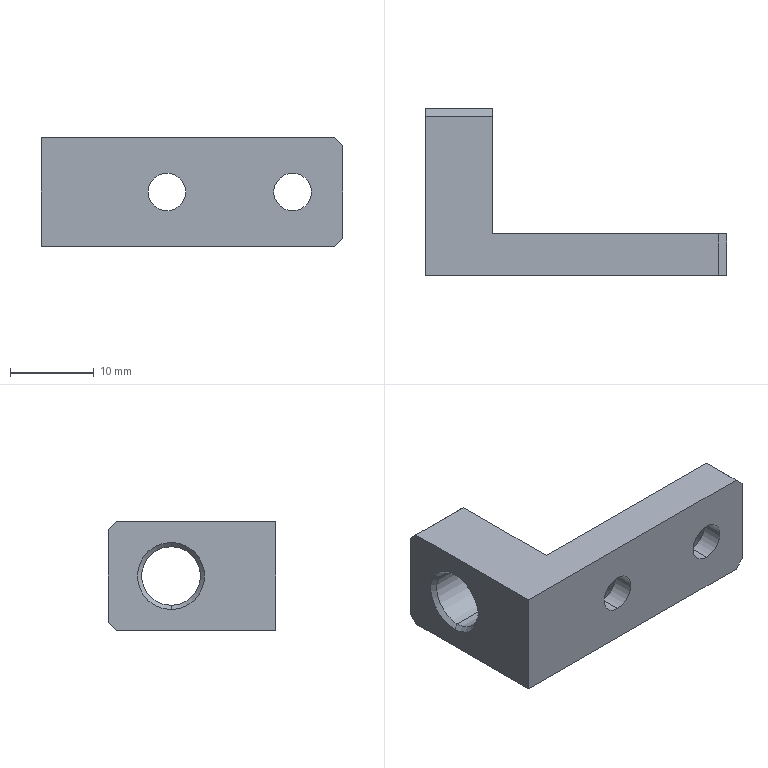Part | STEP file | PN_0073 Mount electronic clip s longitudinal manipulator buffer seat | 1 solid | 26 faces | box 36 x 20 x 13 mm | volume 3299 mm3 | plane 12 | cone 8 | cylinder 6 | commonest cylinder face diameters 4.5 x4 7 x2